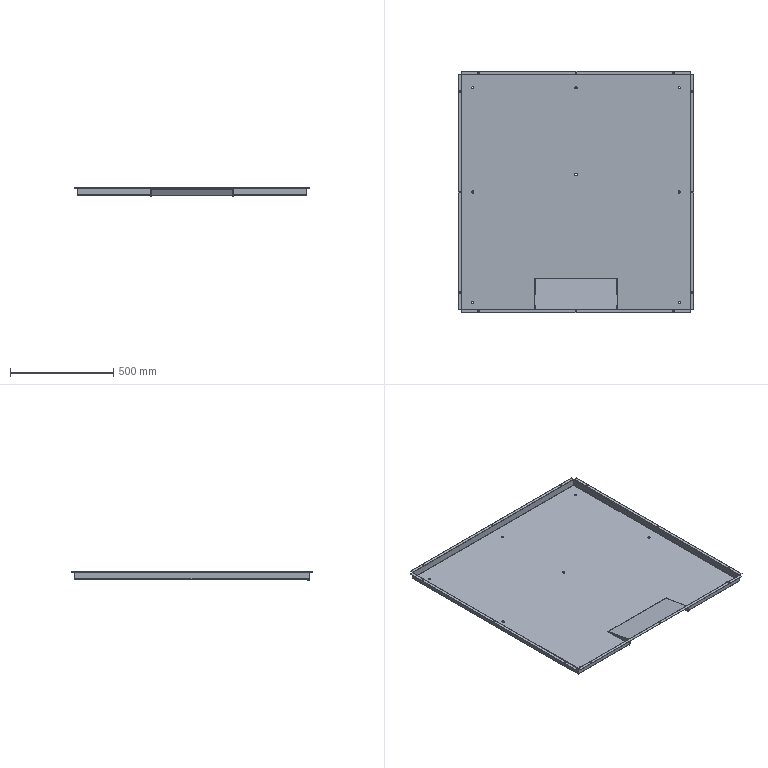Part | 2 solids | 170 faces | box 1140 x 1170 x 39.595 mm | volume 1475814 mm3 | plane 90 | cylinder 68 | spline 12 | commonest cylinder face diameters 7 x30 11 x16 0.4 x9 2.4 x9 2 x2 4 x2